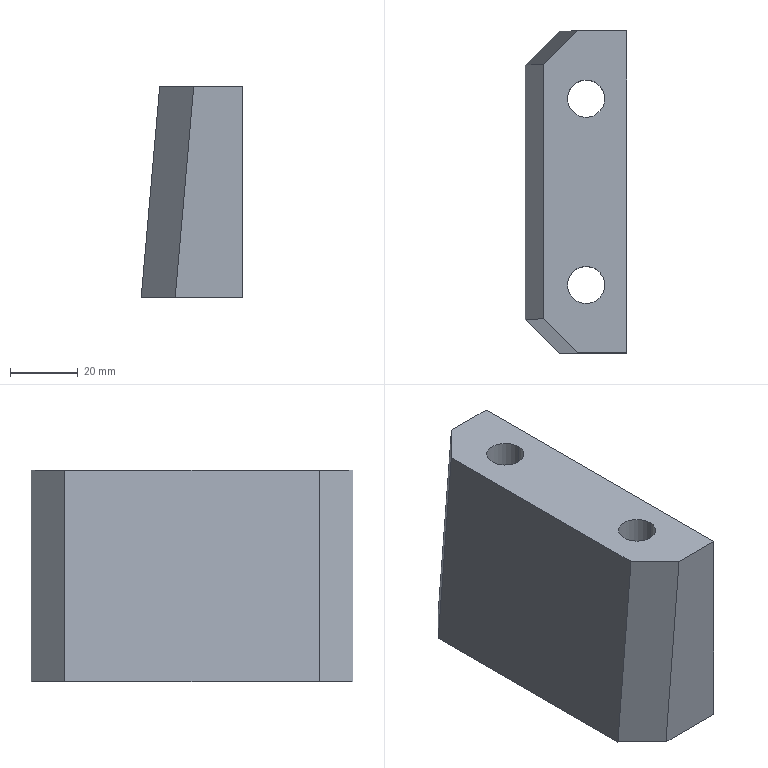Part | Creo | 1 solid | 139 faces | box 30 x 95 x 62.5 mm | volume 138358 mm3 | other 84 | plane 41 | cylinder 12 | cone 2 | commonest cylinder face diameters 11 x4 18 x4 8.5 x2 1.161 x1 2.014 x1